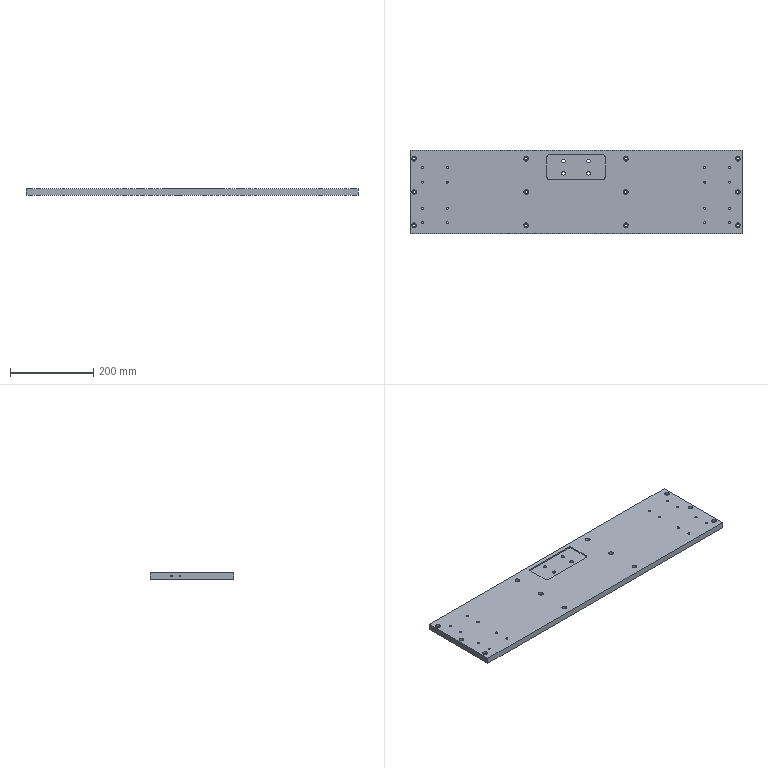Part | STEP file | 0244_212_Plate | 1 solid | 139 faces | box 800 x 200 x 15 mm | volume 2353500 mm3 | cylinder 104 | plane 23 | cone 12 | commonest cylinder face diameters 5 x40 6.6 x24 11 x24 8.5 x8 3.3 x4 10 x4